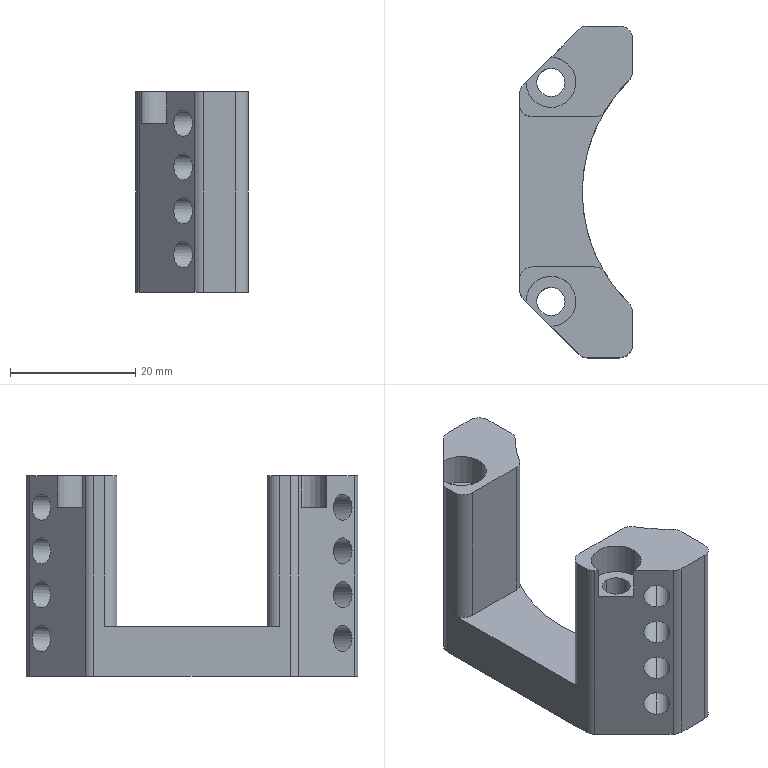NC program | Mastercam | posted with a generic post
Lines 12930 to 13821 of 15624:
N610 T4 M6
N620 G0 G90 G17 G54 X-2.705 Y3.331 A0. S7000 M3
N630 G43 H4 Z50. M8
N640 Z1.
N650 G1 Z.192 F600.
N660 G2 X-.512 Y3.502 Z.122 I3.966 J-36.607 F3000.
N670 X0. Y3.523 Z.106 I1.773 J-36.778
N680 X1.687 Y3.427 Z.053 I-1.261 J-36.799
N690 X3.874 Y3.185 Z-.016 I-2.948 J-36.703
N700 X6.042 Y2.813 Z-.085 I-5.135 J-36.461
N710 X8.185 Y2.313 Z-.154 I-7.303 J-36.089
N720 X9.962 Y1.793 Z-.212 I-9.446 J-35.589
N730 X10.288 Y1.667 Z-.223 I-11.5 J-30.222
N740 X12.307 Y.793 Z-.293 I-11.826 J-30.096
N750 G3 X12.471 Y.756 I.164 J.348
N760 X12.856 Y1.141 I0. J.385
N770 X12.781 Y1.37 I-.385 J0.
N780 G1 X12.532 Y1.707
N790 G2 X12.456 Y1.936 I.309 J.229
N800 X12.841 Y2.321 I.385 J0.
N810 X13.012 Y2.281 I0. J-.385
N820 G1 X15.833 Y.888
N830 X13.929 Y2.792
N840 X11.976
N850 X13.012 Y2.281
N860 G0 Z50.
N870 X2.269 Y4.469
N880 Z1.
N890 G1 Z.192 F600.
N900 X.069 Z.122 F3000.
N910 X-2.131 Z.053
N920 X-4.331 Z-.016
N930 X-6.531 Z-.085
N940 X-8.731 Z-.154
N950 X-10.931 Z-.223
N960 X-13.131 Z-.293
N970 G3 X-13.516 Y4.084 I0. J-.385
N980 X-13.334 Y3.757 I.385 J0.
N990 G1 X-12.928 Y3.504
N1000 G2 X-12.746 Y3.177 I-.203 J-.327
N1010 X-13.131 Y2.792 I-.385 J0.
N1020 G1 X-13.929
N1030 X-15.833 Y.888
N1040 X-11.976 Y2.792
N1050 X-13.131
N1060 G2 X-13.492 Y3.044 I0. J.385
N1070 G1 X-13.925 Y4.217
N1080 G3 X-14.286 Y4.469 I-.361 J-.133
N1090 G1 X-14.623
N1100 X-21.969 Y-2.877
N1110 Y-4.469
N1120 X-20.177
N1130 G2 X-9.962 Y1.793 I21.715 J-23.96
N1140 X0. Y3.523 I11.223 J-35.069
N1150 X9.962 Y1.793 I-1.261 J-36.799
N1160 X20.177 Y-4.469 I-11.5 J-30.222
N1170 G1 X21.969
N1180 Y-2.877
N1190 X14.623 Y4.469
N1200 X-14.286
N1210 G2 X-14.662 Y4.774 I0. J.385
N1220 G1 X-15.049 Y6.592
N1230 G3 X-15.426 Y6.897 I-.377 J-.081
N1240 X-15.441 Y6.896 I0. J-.386
N1250 G1 X-15.624 Y6.889
N1260 X-15.695 Y6.835
N1270 X-24.388 Y-1.874
N1280 X-24.4 Y-6.845
N1290 X-24.391 Y-6.892
N1300 X-24.237 Y-6.9
N1310 X-19.23 Y-6.889
N1320 X-17.536 Y-5.339
N1330 G2 X-15.343 Y-3.675 I46.101 J-58.477
N1340 X-9.561 Y-.651 I15.185 J-21.999
N1350 X-.009 Y1.092 I9.552 J-25.297
N1360 G1 X0.
N1370 X.009
N1380 G2 X9.561 Y-.651 I0. J-27.04
N1390 X15.343 Y-3.675 I-9.403 J-25.023
N1400 X17.536 Y-5.339 I-43.908 J-60.141
N1410 G1 X19.23 Y-6.889
N1420 X24.237 Y-6.9
N1430 X24.391 Y-6.892
N1440 X24.4 Y-6.845
N1450 Y-1.993
N1460 X24.388 Y-1.874
N1470 X24.31 Y-1.78
N1480 X15.626 Y6.888
N1490 X15.343 Y6.9
N1500 X-15.343
N1510 X-15.441 Y6.896
N1520 G0 Z50.
N1530 X-2.705 Y3.331
N1540 Z.707
N1550 G1 Z-.101 F600.
N1560 G2 X-.512 Y3.502 Z-.17 I3.966 J-36.607 F3000.
N1570 X0. Y3.523 Z-.186 I1.773 J-36.778
N1580 X1.687 Y3.427 Z-.239 I-1.261 J-36.799
N1590 X3.874 Y3.185 Z-.308 I-2.948 J-36.703
N1600 X6.042 Y2.813 Z-.378 I-5.135 J-36.461
N1610 X8.185 Y2.313 Z-.447 I-7.303 J-36.089
N1620 X9.962 Y1.793 Z-.505 I-9.446 J-35.589
N1630 X10.288 Y1.667 Z-.516 I-11.5 J-30.222
N1640 X12.307 Y.793 Z-.585 I-11.826 J-30.096
N1650 G3 X12.471 Y.756 I.164 J.348
N1660 X12.856 Y1.141 I0. J.385
N1670 X12.781 Y1.37 I-.385 J0.
N1680 G1 X12.532 Y1.707
N1690 G2 X12.456 Y1.936 I.309 J.229
N1700 X12.841 Y2.321 I.385 J0.
N1710 X13.012 Y2.281 I0. J-.385
N1720 G1 X15.833 Y.888
N1730 X13.929 Y2.792
N1740 X11.976
N1750 X13.012 Y2.281
N1760 G0 Z50.
N1770 X2.269 Y4.469
N1780 Z.707
N1790 G1 Z-.101 F600.
N1800 X.069 Z-.17 F3000.
N1810 X-2.131 Z-.239
N1820 X-4.331 Z-.308
N1830 X-6.531 Z-.378
N1840 X-8.731 Z-.447
N1850 X-10.931 Z-.516
N1860 X-13.131 Z-.585
N1870 G3 X-13.516 Y4.084 I0. J-.385
N1880 X-13.334 Y3.757 I.385 J0.
N1890 G1 X-12.928 Y3.504
N1900 G2 X-12.746 Y3.177 I-.203 J-.327
N1910 X-13.131 Y2.792 I-.385 J0.
N1920 G1 X-13.929
N1930 X-15.833 Y.888
N1940 X-11.976 Y2.792
N1950 X-13.131
N1960 G2 X-13.492 Y3.044 I0. J.385
N1970 G1 X-13.925 Y4.217
N1980 G3 X-14.286 Y4.469 I-.361 J-.133
N1990 G1 X-14.623
N2000 X-21.969 Y-2.877
N2010 Y-4.469
N2020 X-20.177
N2030 G2 X-9.962 Y1.793 I21.715 J-23.96
N2040 X0. Y3.523 I11.223 J-35.069
N2050 X9.962 Y1.793 I-1.261 J-36.799
N2060 X20.177 Y-4.469 I-11.5 J-30.222
N2070 G1 X21.969
N2080 Y-2.877
N2090 X14.623 Y4.469
N2100 X-14.286
N2110 G2 X-14.662 Y4.774 I0. J.385
N2120 G1 X-15.049 Y6.592
N2130 G3 X-15.426 Y6.897 I-.377 J-.081
N2140 X-15.441 Y6.896 I0. J-.386
N2150 G1 X-15.624 Y6.889
N2160 X-15.695 Y6.835
N2170 X-24.388 Y-1.874
N2180 X-24.4 Y-6.845
N2190 X-24.391 Y-6.892
N2200 X-24.237 Y-6.9
N2210 X-19.23 Y-6.889
N2220 X-17.536 Y-5.339
N2230 G2 X-15.343 Y-3.675 I46.101 J-58.477
N2240 X-9.561 Y-.651 I15.185 J-21.999
N2250 X-.009 Y1.092 I9.552 J-25.297
N2260 G1 X0.
N2270 X.009
N2280 G2 X9.561 Y-.651 I0. J-27.04
N2290 X15.343 Y-3.675 I-9.403 J-25.023
N2300 X17.536 Y-5.339 I-43.908 J-60.141
N2310 G1 X19.23 Y-6.889
N2320 X24.237 Y-6.9
N2330 X24.391 Y-6.892
N2340 X24.4 Y-6.845
N2350 Y-1.993
N2360 X24.388 Y-1.874
N2370 X24.31 Y-1.78
N2380 X15.626 Y6.888
N2390 X15.343 Y6.9
N2400 X-15.343
N2410 X-15.441 Y6.896
N2420 G0 Z50.
N2430 X-2.705 Y3.331
N2440 Z.415
N2450 G1 Z-.394 F600.
N2460 G2 X-.512 Y3.502 Z-.463 I3.966 J-36.607 F3000.
N2470 X0. Y3.523 Z-.479 I1.773 J-36.778
N2480 X1.687 Y3.427 Z-.532 I-1.261 J-36.799
N2490 X3.874 Y3.185 Z-.601 I-2.948 J-36.703
N2500 X6.042 Y2.813 Z-.67 I-5.135 J-36.461
N2510 X8.185 Y2.313 Z-.739 I-7.303 J-36.089
N2520 X9.962 Y1.793 Z-.798 I-9.446 J-35.589
N2530 X10.288 Y1.667 Z-.809 I-11.5 J-30.222
N2540 X12.307 Y.793 Z-.878 I-11.826 J-30.096
N2550 G3 X12.471 Y.756 I.164 J.348
N2560 X12.856 Y1.141 I0. J.385
N2570 X12.781 Y1.37 I-.385 J0.
N2580 G1 X12.532 Y1.707
N2590 G2 X12.456 Y1.936 I.309 J.229
N2600 X12.841 Y2.321 I.385 J0.
N2610 X13.012 Y2.281 I0. J-.385
N2620 G1 X15.833 Y.888
N2630 X13.929 Y2.792
N2640 X11.976
N2650 X13.012 Y2.281
N2660 G0 Z50.
N2670 X2.269 Y4.469
N2680 Z.415
N2690 G1 Z-.394 F600.
N2700 X.069 Z-.463 F3000.
N2710 X-2.131 Z-.532
N2720 X-4.331 Z-.601
N2730 X-6.531 Z-.67
N2740 X-8.731 Z-.739
N2750 X-10.931 Z-.809
N2760 X-13.131 Z-.878
N2770 G3 X-13.516 Y4.084 I0. J-.385
N2780 X-13.334 Y3.757 I.385 J0.
N2790 G1 X-12.928 Y3.504
N2800 G2 X-12.746 Y3.177 I-.203 J-.327
N2810 X-13.131 Y2.792 I-.385 J0.
N2820 G1 X-13.929
N2830 X-15.833 Y.888
N2840 X-11.976 Y2.792
N2850 X-13.131
N2860 G2 X-13.492 Y3.044 I0. J.385
N2870 G1 X-13.925 Y4.217
N2880 G3 X-14.286 Y4.469 I-.361 J-.133
N2890 G1 X-14.623
N2900 X-21.969 Y-2.877
N2910 Y-4.469
N2920 X-20.177
N2930 G2 X-9.962 Y1.793 I21.715 J-23.96
N2940 X0. Y3.523 I11.223 J-35.069
N2950 X9.962 Y1.793 I-1.261 J-36.799
N2960 X20.177 Y-4.469 I-11.5 J-30.222
N2970 G1 X21.969
N2980 Y-2.877
N2990 X14.623 Y4.469
N3000 X-14.286
N3010 G2 X-14.662 Y4.774 I0. J.385
N3020 G1 X-15.049 Y6.592
N3030 G3 X-15.426 Y6.897 I-.377 J-.081
N3040 X-15.441 Y6.896 I0. J-.386
N3050 G1 X-15.624 Y6.889
N3060 X-15.695 Y6.835
N3070 X-24.388 Y-1.874
N3080 X-24.4 Y-6.845
N3090 X-24.391 Y-6.892
N3100 X-24.237 Y-6.9
N3110 X-19.23 Y-6.889
N3120 X-17.536 Y-5.339
N3130 G2 X-15.343 Y-3.675 I46.101 J-58.477
N3140 X-9.561 Y-.651 I15.185 J-21.999
N3150 X-.009 Y1.092 I9.552 J-25.297
N3160 G1 X0.
N3170 X.009
N3180 G2 X9.561 Y-.651 I0. J-27.04
N3190 X15.343 Y-3.675 I-9.403 J-25.023
N3200 X17.536 Y-5.339 I-43.908 J-60.141
N3210 G1 X19.23 Y-6.889
N3220 X24.237 Y-6.9
N3230 X24.391 Y-6.892
N3240 X24.4 Y-6.845
N3250 Y-1.993
N3260 X24.388 Y-1.874
N3270 X24.31 Y-1.78
N3280 X15.626 Y6.888
N3290 X15.343 Y6.9
N3300 X-15.343
N3310 X-15.441 Y6.896
N3320 G0 Z50.
N3330 X-2.705 Y3.331
N3340 Z.122
N3350 G1 Z-.686 F600.
N3360 G2 X-.512 Y3.502 Z-.755 I3.966 J-36.607 F3000.
N3370 X0. Y3.523 Z-.771 I1.773 J-36.778
N3380 X1.687 Y3.427 Z-.824 I-1.261 J-36.799
N3390 X3.874 Y3.185 Z-.894 I-2.948 J-36.703
N3400 X6.042 Y2.813 Z-.963 I-5.135 J-36.461
N3410 X8.185 Y2.313 Z-1.032 I-7.303 J-36.089
N3420 X9.962 Y1.793 Z-1.09 I-9.446 J-35.589
N3430 X10.288 Y1.667 Z-1.101 I-11.5 J-30.222
N3440 X12.307 Y.793 Z-1.17 I-11.826 J-30.096
N3450 G3 X12.471 Y.756 I.164 J.348
N3460 X12.856 Y1.141 I0. J.385
N3470 X12.781 Y1.37 I-.385 J0.
N3480 G1 X12.532 Y1.707
N3490 G2 X12.456 Y1.936 I.309 J.229
N3500 X12.841 Y2.321 I.385 J0.
N3510 X13.012 Y2.281 I0. J-.385
N3520 G1 X15.833 Y.888
N3530 X13.929 Y2.792
N3540 X11.976
N3550 X13.012 Y2.281
N3560 G0 Z50.
N3570 X2.269 Y4.469
N3580 Z.122
N3590 G1 Z-.686 F600.
N3600 X.069 Z-.755 F3000.
N3610 X-2.131 Z-.824
N3620 X-4.331 Z-.894
N3630 X-6.531 Z-.963
N3640 X-8.731 Z-1.032
N3650 X-10.931 Z-1.101
N3660 X-13.131 Z-1.17
N3670 G3 X-13.516 Y4.084 I0. J-.385
N3680 X-13.334 Y3.757 I.385 J0.
N3690 G1 X-12.928 Y3.504
N3700 G2 X-12.746 Y3.177 I-.203 J-.327
N3710 X-13.131 Y2.792 I-.385 J0.
N3720 G1 X-13.929
N3730 X-15.833 Y.888
N3740 X-11.976 Y2.792
N3750 X-13.131
N3760 G2 X-13.492 Y3.044 I0. J.385
N3770 G1 X-13.925 Y4.217
N3780 G3 X-14.286 Y4.469 I-.361 J-.133
N3790 G1 X-14.623
N3800 X-21.969 Y-2.877
N3810 Y-4.469
N3820 X-20.177
N3830 G2 X-9.962 Y1.793 I21.715 J-23.96
N3840 X0. Y3.523 I11.223 J-35.069
N3850 X9.962 Y1.793 I-1.261 J-36.799
N3860 X20.177 Y-4.469 I-11.5 J-30.222
N3870 G1 X21.969
N3880 Y-2.877
N3890 X14.623 Y4.469
N3900 X-14.286
N3910 G2 X-14.662 Y4.774 I0. J.385
N3920 G1 X-15.049 Y6.592
N3930 G3 X-15.426 Y6.897 I-.377 J-.081
N3940 X-15.441 Y6.896 I0. J-.386
N3950 G1 X-15.624 Y6.889
N3960 X-15.695 Y6.835
N3970 X-24.388 Y-1.874
N3980 X-24.4 Y-6.845
N3990 X-24.391 Y-6.892
N4000 X-24.237 Y-6.9
N4010 X-19.23 Y-6.889
N4020 X-17.536 Y-5.339
N4030 G2 X-15.343 Y-3.675 I46.101 J-58.477
N4040 X-9.561 Y-.651 I15.185 J-21.999
N4050 X-.009 Y1.092 I9.552 J-25.297
N4060 G1 X0.
N4070 X.009
N4080 G2 X9.561 Y-.651 I0. J-27.04
N4090 X15.343 Y-3.675 I-9.403 J-25.023
N4100 X17.536 Y-5.339 I-43.908 J-60.141
N4110 G1 X19.23 Y-6.889
N4120 X24.237 Y-6.9
N4130 X24.391 Y-6.892
N4140 X24.4 Y-6.845
N4150 Y-1.993
N4160 X24.388 Y-1.874
N4170 X24.31 Y-1.78
N4180 X15.626 Y6.888
N4190 X15.343 Y6.9
N4200 X-15.343
N4210 X-15.441 Y6.896
N4220 G0 Z50.
N4230 X-2.705 Y3.331
N4240 Z-.17
N4250 G1 Z-.979 F600.
N4260 G2 X-.512 Y3.502 Z-1.048 I3.966 J-36.607 F3000.
N4270 X0. Y3.523 Z-1.064 I1.773 J-36.778
N4280 X1.687 Y3.427 Z-1.117 I-1.261 J-36.799
N4290 X3.874 Y3.185 Z-1.186 I-2.948 J-36.703
N4300 X6.042 Y2.813 Z-1.255 I-5.135 J-36.461
N4310 X8.185 Y2.313 Z-1.325 I-7.303 J-36.089
N4320 X9.962 Y1.793 Z-1.383 I-9.446 J-35.589
N4330 X10.288 Y1.667 Z-1.394 I-11.5 J-30.222
N4340 X12.307 Y.793 Z-1.463 I-11.826 J-30.096
N4350 G3 X12.471 Y.756 I.164 J.348
N4360 X12.856 Y1.141 I0. J.385
N4370 X12.781 Y1.37 I-.385 J0.
N4380 G1 X12.532 Y1.707
N4390 G2 X12.456 Y1.936 I.309 J.229
N4400 X12.841 Y2.321 I.385 J0.
N4410 X13.012 Y2.281 I0. J-.385
N4420 G1 X15.833 Y.888
N4430 X13.929 Y2.792
N4440 X11.976
N4450 X13.012 Y2.281
N4460 G0 Z50.
N4470 X2.269 Y4.469
N4480 Z-.17
N4490 G1 Z-.979 F600.
N4500 X.069 Z-1.048 F3000.
N4510 X-2.131 Z-1.117
N4520 X-4.331 Z-1.186
N4530 X-6.531 Z-1.255
N4540 X-8.731 Z-1.325
N4550 X-10.931 Z-1.394
N4560 X-13.131 Z-1.463
N4570 G3 X-13.516 Y4.084 I0. J-.385
N4580 X-13.334 Y3.757 I.385 J0.
N4590 G1 X-12.928 Y3.504
N4600 G2 X-12.746 Y3.177 I-.203 J-.327
N4610 X-13.131 Y2.792 I-.385 J0.
N4620 G1 X-13.929
N4630 X-15.833 Y.888
N4640 X-11.976 Y2.792
N4650 X-13.131
N4660 G2 X-13.492 Y3.044 I0. J.385
N4670 G1 X-13.925 Y4.217
N4680 G3 X-14.286 Y4.469 I-.361 J-.133
N4690 G1 X-14.623
N4700 X-21.969 Y-2.877
N4710 Y-4.469
N4720 X-20.177
N4730 G2 X-9.962 Y1.793 I21.715 J-23.96
N4740 X0. Y3.523 I11.223 J-35.069
N4750 X9.962 Y1.793 I-1.261 J-36.799
N4760 X20.177 Y-4.469 I-11.5 J-30.222
N4770 G1 X21.969
N4780 Y-2.877
N4790 X14.623 Y4.469
N4800 X-14.286
N4810 G2 X-14.662 Y4.774 I0. J.385
N4820 G1 X-15.049 Y6.592
N4830 G3 X-15.426 Y6.897 I-.377 J-.081
N4840 X-15.441 Y6.896 I0. J-.386
N4850 G1 X-15.624 Y6.889
N4860 X-15.695 Y6.835
N4870 X-24.388 Y-1.874
N4880 X-24.4 Y-6.845
N4890 X-24.391 Y-6.892
N4900 X-24.237 Y-6.9
N4910 X-19.23 Y-6.889
N4920 X-17.536 Y-5.339
N4930 G2 X-15.343 Y-3.675 I46.101 J-58.477
N4940 X-9.561 Y-.651 I15.185 J-21.999
N4950 X-.009 Y1.092 I9.552 J-25.297
N4960 G1 X0.
N4970 X.009
N4980 G2 X9.561 Y-.651 I0. J-27.04
N4990 X15.343 Y-3.675 I-9.403 J-25.023
N5000 X17.536 Y-5.339 I-43.908 J-60.141
N5010 G1 X19.23 Y-6.889
N5020 X24.237 Y-6.9
N5030 X24.391 Y-6.892
N5040 X24.4 Y-6.845
N5050 Y-1.993
N5060 X24.388 Y-1.874
N5070 X24.31 Y-1.78
N5080 X15.626 Y6.888
N5090 X15.343 Y6.9
N5100 X-15.343
N5110 X-15.441 Y6.896
N5120 G0 Z50.
N5130 X-2.705 Y3.331
N5140 Z-.463
N5150 G1 Z-1.271 F600.
N5160 G2 X-.512 Y3.502 Z-1.34 I3.966 J-36.607 F3000.
N5170 X0. Y3.523 Z-1.357 I1.773 J-36.778
N5180 X1.687 Y3.427 Z-1.41 I-1.261 J-36.799
N5190 X3.874 Y3.185 Z-1.479 I-2.948 J-36.703
N5200 X6.042 Y2.813 Z-1.548 I-5.135 J-36.461
N5210 X8.185 Y2.313 Z-1.617 I-7.303 J-36.089
N5220 X9.962 Y1.793 Z-1.675 I-9.446 J-35.589
N5230 X10.288 Y1.667 Z-1.686 I-11.5 J-30.222
N5240 X12.307 Y.793 Z-1.756 I-11.826 J-30.096
N5250 G3 X12.471 Y.756 I.164 J.348
N5260 X12.856 Y1.141 I0. J.385
N5270 X12.781 Y1.37 I-.385 J0.
N5280 G1 X12.532 Y1.707
N5290 G2 X12.456 Y1.936 I.309 J.229
N5300 X12.841 Y2.321 I.385 J0.
N5310 X13.012 Y2.281 I0. J-.385
N5320 G1 X15.833 Y.888
N5330 X13.929 Y2.792
N5340 X11.976
N5350 X13.012 Y2.281
N5360 G0 Z50.
N5370 X2.269 Y4.469
N5380 Z-.463
N5390 G1 Z-1.271 F600.
N5400 X.069 Z-1.34 F3000.
N5410 X-2.131 Z-1.41
N5420 X-4.331 Z-1.479
N5430 X-6.531 Z-1.548
N5440 X-8.731 Z-1.617
N5450 X-10.931 Z-1.686
N5460 X-13.131 Z-1.756
N5470 G3 X-13.516 Y4.084 I0. J-.385
N5480 X-13.334 Y3.757 I.385 J0.
N5490 G1 X-12.928 Y3.504
N5500 G2 X-12.746 Y3.177 I-.203 J-.327
N5510 X-13.131 Y2.792 I-.385 J0.
N5520 G1 X-13.929
N5530 X-15.833 Y.888
N5540 X-11.976 Y2.792
N5550 X-13.131
N5560 G2 X-13.492 Y3.044 I0. J.385
N5570 G1 X-13.925 Y4.217
N5580 G3 X-14.286 Y4.469 I-.361 J-.133
N5590 G1 X-14.623
N5600 X-21.969 Y-2.877
N5610 Y-4.469
N5620 X-20.177
N5630 G2 X-9.962 Y1.793 I21.715 J-23.96
N5640 X0. Y3.523 I11.223 J-35.069
N5650 X9.962 Y1.793 I-1.261 J-36.799
N5660 X20.177 Y-4.469 I-11.5 J-30.222
N5670 G1 X21.969
N5680 Y-2.877
N5690 X14.623 Y4.469
N5700 X-14.286
N5710 G2 X-14.662 Y4.774 I0. J.385
N5720 G1 X-15.049 Y6.592
N5730 G3 X-15.426 Y6.897 I-.377 J-.081
N5740 X-15.441 Y6.896 I0. J-.386
N5750 G1 X-15.624 Y6.889
N5760 X-15.695 Y6.835
N5770 X-24.388 Y-1.874
N5780 X-24.4 Y-6.845
N5790 X-24.391 Y-6.892
N5800 X-24.237 Y-6.9
N5810 X-19.23 Y-6.889
N5820 X-17.536 Y-5.339
N5830 G2 X-15.343 Y-3.675 I46.101 J-58.477
N5840 X-9.561 Y-.651 I15.185 J-21.999
N5850 X-.009 Y1.092 I9.552 J-25.297
N5860 G1 X0.
N5870 X.009
N5880 G2 X9.561 Y-.651 I0. J-27.04
N5890 X15.343 Y-3.675 I-9.403 J-25.023
N5900 X17.536 Y-5.339 I-43.908 J-60.141
N5910 G1 X19.23 Y-6.889
N5920 X24.237 Y-6.9
N5930 X24.391 Y-6.892
N5940 X24.4 Y-6.845
N5950 Y-1.993
N5960 X24.388 Y-1.874
N5970 X24.31 Y-1.78
N5980 X15.626 Y6.888
N5990 X15.343 Y6.9
N6000 X-15.343
N6010 X-15.441 Y6.896
N6020 G0 Z50.
N6030 X-2.705 Y3.331
N6040 Z-.756
N6050 G1 Z-1.564 F600.
N6060 G2 X-.512 Y3.502 Z-1.633 I3.966 J-36.607 F3000.
N6070 X0. Y3.523 Z-1.649 I1.773 J-36.778
N6080 X1.687 Y3.427 Z-1.702 I-1.261 J-36.799
N6090 X3.874 Y3.185 Z-1.771 I-2.948 J-36.703
N6100 X6.042 Y2.813 Z-1.841 I-5.135 J-36.461
N6110 X8.185 Y2.313 Z-1.91 I-7.303 J-36.089
N6120 X9.962 Y1.793 Z-1.968 I-9.446 J-35.589
N6130 X10.288 Y1.667 Z-1.979 I-11.5 J-30.222
N6140 X12.307 Y.793 Z-2.048 I-11.826 J-30.096
N6150 G3 X12.471 Y.756 I.164 J.348
N6160 X12.856 Y1.141 I0. J.385
N6170 X12.781 Y1.37 I-.385 J0.
N6180 G1 X12.532 Y1.707
N6190 G2 X12.456 Y1.936 I.309 J.229
N6200 X12.841 Y2.321 I.385 J0.
N6210 X13.012 Y2.281 I0. J-.385
N6220 G1 X15.833 Y.888
N6230 X13.929 Y2.792
N6240 X11.976
N6250 X13.012 Y2.281
N6260 G0 Z50.
N6270 X2.269 Y4.469
N6280 Z-.756
N6290 G1 Z-1.564 F600.
N6300 X.069 Z-1.633 F3000.
N6310 X-2.131 Z-1.702
N6320 X-4.331 Z-1.771
N6330 X-6.531 Z-1.841
N6340 X-8.731 Z-1.91
N6350 X-10.931 Z-1.979
N6360 X-13.131 Z-2.048
N6370 G3 X-13.516 Y4.084 I0. J-.385
N6380 X-13.334 Y3.757 I.385 J0.
N6390 G1 X-12.928 Y3.504
N6400 G2 X-12.746 Y3.177 I-.203 J-.327
N6410 X-13.131 Y2.792 I-.385 J0.
N6420 G1 X-13.929
N6430 X-15.833 Y.888
N6440 X-11.976 Y2.792
N6450 X-13.131
N6460 G2 X-13.492 Y3.044 I0. J.385
N6470 G1 X-13.925 Y4.217
N6480 G3 X-14.286 Y4.469 I-.361 J-.133
N6490 G1 X-14.623
N6500 X-21.969 Y-2.877
N6510 Y-4.469
N6520 X-20.177
N6530 G2 X-9.962 Y1.793 I21.715 J-23.96
N6540 X0. Y3.523 I11.223 J-35.069
N6550 X9.962 Y1.793 I-1.261 J-36.799
N6560 X20.177 Y-4.469 I-11.5 J-30.222
N6570 G1 X21.969
N6580 Y-2.877
N6590 X14.623 Y4.469
N6600 X-14.286
N6610 G2 X-14.662 Y4.774 I0. J.385
N6620 G1 X-15.049 Y6.592
N6630 G3 X-15.426 Y6.897 I-.377 J-.081
N6640 X-15.441 Y6.896 I0. J-.386
N6650 G1 X-15.624 Y6.889
N6660 X-15.695 Y6.835
N6670 X-24.388 Y-1.874
N6680 X-24.4 Y-6.845
N6690 X-24.391 Y-6.892
N6700 X-24.237 Y-6.9
N6710 X-19.23 Y-6.889
N6720 X-17.536 Y-5.339
N6730 G2 X-15.343 Y-3.675 I46.101 J-58.477
N6740 X-9.561 Y-.651 I15.185 J-21.999
N6750 X-.009 Y1.092 I9.552 J-25.297
N6760 G1 X0.
N6770 X.009
N6780 G2 X9.561 Y-.651 I0. J-27.04
N6790 X15.343 Y-3.675 I-9.403 J-25.023
N6800 X17.536 Y-5.339 I-43.908 J-60.141
N6810 G1 X19.23 Y-6.889
N6820 X24.237 Y-6.9
N6830 X24.391 Y-6.892
N6840 X24.4 Y-6.845
N6850 Y-1.993
N6860 X24.388 Y-1.874
N6870 X24.31 Y-1.78
N6880 X15.626 Y6.888
N6890 X15.343 Y6.9
N6900 X-15.343
N6910 X-15.441 Y6.896
N6920 G0 Z50.
N6930 X-2.705 Y3.331
N6940 Z-1.048
N6950 G1 Z-1.856 F600.
N6960 G2 X-.512 Y3.502 Z-1.926 I3.966 J-36.607 F3000.
N6970 X0. Y3.523 Z-1.942 I1.773 J-36.778
N6980 X1.687 Y3.427 Z-1.995 I-1.261 J-36.799
N6990 X3.874 Y3.185 Z-2.064 I-2.948 J-36.703
N7000 X6.042 Y2.813 Z-2.133 I-5.135 J-36.461
N7010 X8.185 Y2.313 Z-2.202 I-7.303 J-36.089
N7020 X9.962 Y1.793 Z-2.261 I-9.446 J-35.589
N7030 X10.288 Y1.667 Z-2.272 I-11.5 J-30.222
N7040 X12.307 Y.793 Z-2.341 I-11.826 J-30.096
N7050 G3 X12.471 Y.756 I.164 J.348
N7060 X12.856 Y1.141 I0. J.385
N7070 X12.781 Y1.37 I-.385 J0.
N7080 G1 X12.532 Y1.707
N7090 G2 X12.456 Y1.936 I.309 J.229
N7100 X12.841 Y2.321 I.385 J0.
N7110 X13.012 Y2.281 I0. J-.385
N7120 G1 X15.833 Y.888
N7130 X13.929 Y2.792
N7140 X11.976
N7150 X13.012 Y2.281
N7160 G0 Z50.
N7170 X2.269 Y4.469
N7180 Z-1.048
N7190 G1 Z-1.856 F600.
N7200 X.069 Z-1.926 F3000.
N7210 X-2.131 Z-1.995
N7220 X-4.331 Z-2.064
N7230 X-6.531 Z-2.133
N7240 X-8.731 Z-2.202
N7250 X-10.931 Z-2.272
N7260 X-13.131 Z-2.341
N7270 G3 X-13.516 Y4.084 I0. J-.385
N7280 X-13.334 Y3.757 I.385 J0.
N7290 G1 X-12.928 Y3.504
N7300 G2 X-12.746 Y3.177 I-.203 J-.327
N7310 X-13.131 Y2.792 I-.385 J0.
N7320 G1 X-13.929
N7330 X-15.833 Y.888
N7340 X-11.976 Y2.792
N7350 X-13.131
N7360 G2 X-13.492 Y3.044 I0. J.385
N7370 G1 X-13.925 Y4.217
N7380 G3 X-14.286 Y4.469 I-.361 J-.133
N7390 G1 X-14.623
N7400 X-21.969 Y-2.877
N7410 Y-4.469
N7420 X-20.177
N7430 G2 X-9.962 Y1.793 I21.715 J-23.96
N7440 X0. Y3.523 I11.223 J-35.069
N7450 X9.962 Y1.793 I-1.261 J-36.799
N7460 X20.177 Y-4.469 I-11.5 J-30.222
N7470 G1 X21.969
N7480 Y-2.877
N7490 X14.623 Y4.469
N7500 X-14.286
N7510 G2 X-14.662 Y4.774 I0. J.385
N7520 G1 X-15.049 Y6.592
N7530 G3 X-15.426 Y6.897 I-.377 J-.081
N7540 X-15.441 Y6.896 I0. J-.386
N7550 G1 X-15.624 Y6.889
N7560 X-15.695 Y6.835
N7570 X-24.388 Y-1.874
N7580 X-24.4 Y-6.845
N7590 X-24.391 Y-6.892
N7600 X-24.237 Y-6.9
N7610 X-19.23 Y-6.889
N7620 X-17.536 Y-5.339
N7630 G2 X-15.343 Y-3.675 I46.101 J-58.477
N7640 X-9.561 Y-.651 I15.185 J-21.999
N7650 X-.009 Y1.092 I9.552 J-25.297
N7660 G1 X0.
N7670 X.009
N7680 G2 X9.561 Y-.651 I0. J-27.04
N7690 X15.343 Y-3.675 I-9.403 J-25.023
N7700 X17.536 Y-5.339 I-43.908 J-60.141
N7710 G1 X19.23 Y-6.889
N7720 X24.237 Y-6.9
N7730 X24.391 Y-6.892
N7740 X24.4 Y-6.845
N7750 Y-1.993
N7760 X24.388 Y-1.874
N7770 X24.31 Y-1.78
N7780 X15.626 Y6.888
N7790 X15.343 Y6.9
N7800 X-15.343
N7810 X-15.441 Y6.896
N7820 G0 Z50.
N7830 X-2.705 Y3.331
N7840 Z-1.341
N7850 G1 Z-2.149 F600.
N7860 G2 X-.512 Y3.502 Z-2.218 I3.966 J-36.607 F3000.
N7870 X0. Y3.523 Z-2.234 I1.773 J-36.778
N7880 X1.687 Y3.427 Z-2.287 I-1.261 J-36.799
N7890 X3.874 Y3.185 Z-2.357 I-2.948 J-36.703
N7900 X6.042 Y2.813 Z-2.426 I-5.135 J-36.461
N7910 X8.185 Y2.313 Z-2.495 I-7.303 J-36.089
N7920 X9.962 Y1.793 Z-2.553 I-9.446 J-35.589
N7930 X10.288 Y1.667 Z-2.564 I-11.5 J-30.222
N7940 X12.307 Y.793 Z-2.633 I-11.826 J-30.096
N7950 G3 X12.471 Y.756 I.164 J.348
N7960 X12.856 Y1.141 I0. J.385
N7970 X12.781 Y1.37 I-.385 J0.
N7980 G1 X12.532 Y1.707
N7990 G2 X12.456 Y1.936 I.309 J.229
N8000 X12.841 Y2.321 I.385 J0.
N8010 X13.012 Y2.281 I0. J-.385
N8020 G1 X15.833 Y.888
N8030 X13.929 Y2.792
N8040 X11.976
N8050 X13.012 Y2.281
N8060 G0 Z50.
N8070 X2.269 Y4.469
N8080 Z-1.341
N8090 G1 Z-2.149 F600.
N8100 X.069 Z-2.218 F3000.
N8110 X-2.131 Z-2.287
N8120 X-4.331 Z-2.357
N8130 X-6.531 Z-2.426
N8140 X-8.731 Z-2.495
N8150 X-10.931 Z-2.564
N8160 X-13.131 Z-2.633
N8170 G3 X-13.516 Y4.084 I0. J-.385
N8180 X-13.334 Y3.757 I.385 J0.
N8190 G1 X-12.928 Y3.504
N8200 G2 X-12.746 Y3.177 I-.203 J-.327
N8210 X-13.131 Y2.792 I-.385 J0.
N8220 G1 X-13.929
N8230 X-15.833 Y.888
N8240 X-11.976 Y2.792
N8250 X-13.131
N8260 G2 X-13.492 Y3.044 I0. J.385
N8270 G1 X-13.925 Y4.217
N8280 G3 X-14.286 Y4.469 I-.361 J-.133
N8290 G1 X-14.623
N8300 X-21.969 Y-2.877
N8310 Y-4.469
N8320 X-20.177
N8330 G2 X-9.962 Y1.793 I21.715 J-23.96
N8340 X0. Y3.523 I11.223 J-35.069
N8350 X9.962 Y1.793 I-1.261 J-36.799
N8360 X20.177 Y-4.469 I-11.5 J-30.222
N8370 G1 X21.969
N8380 Y-2.877
N8390 X14.623 Y4.469
N8400 X-14.286
N8410 G2 X-14.662 Y4.774 I0. J.385
N8420 G1 X-15.049 Y6.592
N8430 G3 X-15.426 Y6.897 I-.377 J-.081
N8440 X-15.441 Y6.896 I0. J-.386
N8450 G1 X-15.624 Y6.889
N8460 X-15.695 Y6.835
N8470 X-24.388 Y-1.874
N8480 X-24.4 Y-6.845
N8490 X-24.391 Y-6.892
N8500 X-24.237 Y-6.9
N8510 X-19.23 Y-6.889
N8520 X-17.536 Y-5.339
N8530 G2 X-15.343 Y-3.675 I46.101 J-58.477
N8540 X-9.561 Y-.651 I15.185 J-21.999
N8550 X-.009 Y1.092 I9.552 J-25.297
N8560 G1 X0.
N8570 X.009
N8580 G2 X9.561 Y-.651 I0. J-27.04
N8590 X15.343 Y-3.675 I-9.403 J-25.023
N8600 X17.536 Y-5.339 I-43.908 J-60.141
N8610 G1 X19.23 Y-6.889
N8620 X24.237 Y-6.9
N8630 X24.391 Y-6.892
N8640 X24.4 Y-6.845
N8650 Y-1.993
N8660 X24.388 Y-1.874
N8670 X24.31 Y-1.78
N8680 X15.626 Y6.888
N8690 X15.343 Y6.9
N8700 X-15.343
N8710 X-15.441 Y6.896
N8720 G0 Z50.
N8730 X-2.705 Y3.331
N8740 Z-1.633
N8750 G1 Z-2.442 F600.
N8760 G2 X-.512 Y3.502 Z-2.511 I3.966 J-36.607 F3000.
N8770 X0. Y3.523 Z-2.527 I1.773 J-36.778
N8780 X1.687 Y3.427 Z-2.58 I-1.261 J-36.799
N8790 X3.874 Y3.185 Z-2.649 I-2.948 J-36.703
N8800 X6.042 Y2.813 Z-2.718 I-5.135 J-36.461
N8810 X8.185 Y2.313 Z-2.788 I-7.303 J-36.089
N8820 X9.962 Y1.793 Z-2.846 I-9.446 J-35.589
N8830 X10.288 Y1.667 Z-2.857 I-11.5 J-30.222
N8840 X12.307 Y.793 Z-2.926 I-11.826 J-30.096
N8850 G3 X12.471 Y.756 I.164 J.348
N8860 X12.856 Y1.141 I0. J.385
N8870 X12.781 Y1.37 I-.385 J0.
N8880 G1 X12.532 Y1.707
N8890 G2 X12.456 Y1.936 I.309 J.229
N8900 X12.841 Y2.321 I.385 J0.
N8910 X13.012 Y2.281 I0. J-.385
N8920 G1 X15.833 Y.888
N8930 X13.929 Y2.792
N8940 X11.976
N8950 X13.012 Y2.281
N8960 G0 Z50.
N8970 X2.269 Y4.469
N8980 Z-1.633
N8990 G1 Z-2.442 F600.
N9000 X.069 Z-2.511 F3000.
N9010 X-2.131 Z-2.58
N9020 X-4.331 Z-2.649
N9030 X-6.531 Z-2.718
N9040 X-8.731 Z-2.788
N9050 X-10.931 Z-2.857
N9060 X-13.131 Z-2.926
N9070 G3 X-13.516 Y4.084 I0. J-.385
N9080 X-13.334 Y3.757 I.385 J0.
N9090 G1 X-12.928 Y3.504
N9100 G2 X-12.746 Y3.177 I-.203 J-.327
N9110 X-13.131 Y2.792 I-.385 J0.
N9120 G1 X-13.929
N9130 X-15.833 Y.888
N9140 X-11.976 Y2.792
N9150 X-13.131
N9160 G2 X-13.492 Y3.044 I0. J.385
N9170 G1 X-13.925 Y4.217
N9180 G3 X-14.286 Y4.469 I-.361 J-.133
N9190 G1 X-14.623
N9200 X-21.969 Y-2.877
N9210 Y-4.469
N9220 X-20.177
N9230 G2 X-9.962 Y1.793 I21.715 J-23.96
N9240 X0. Y3.523 I11.223 J-35.069
N9250 X9.962 Y1.793 I-1.261 J-36.799
N9260 X20.177 Y-4.469 I-11.5 J-30.222
N9270 G1 X21.969
N9280 Y-2.877
N9290 X14.623 Y4.469
N9300 X-14.286
N9310 G2 X-14.662 Y4.774 I0. J.385
N9320 G1 X-15.049 Y6.592
N9330 G3 X-15.426 Y6.897 I-.377 J-.081
N9340 X-15.441 Y6.896 I0. J-.386
N9350 G1 X-15.624 Y6.889
N9360 X-15.695 Y6.835
N9370 X-24.388 Y-1.874
N9380 X-24.4 Y-6.845
N9390 X-24.391 Y-6.892
N9400 X-24.237 Y-6.9
N9410 X-19.23 Y-6.889
N9420 X-17.536 Y-5.339
N9430 G2 X-15.343 Y-3.675 I46.101 J-58.477
N9440 X-9.561 Y-.651 I15.185 J-21.999
N9450 X-.009 Y1.092 I9.552 J-25.297
N9460 G1 X0.
N9470 X.009
N9480 G2 X9.561 Y-.651 I0. J-27.04
N9490 X15.343 Y-3.675 I-9.403 J-25.023
N9500 X17.536 Y-5.339 I-43.908 J-60.141
N9510 G1 X19.23 Y-6.889
N9520 X24.237 Y-6.9